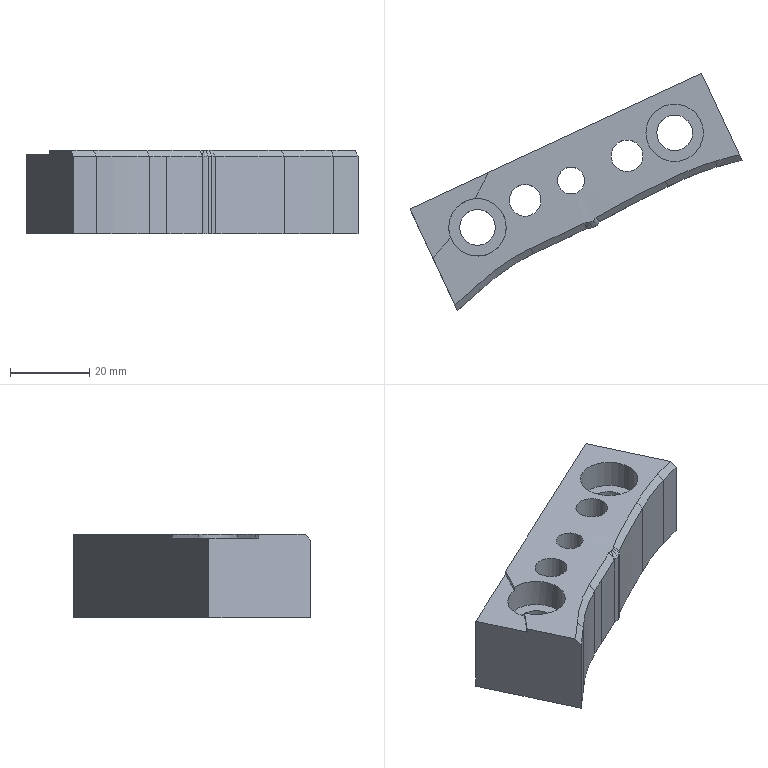Part | NX | features 23 2 | 1 solid | 38 faces | box 83.645 x 59.809 x 21 mm | volume 32912 mm3 | cylinder 17 | plane 10 | cone 9 | spline 2 | commonest cylinder face diameters 4.4 x2 8.001 x2 9 x2 14.5 x2 6.8 x1 134.826 x1
STEP:
#1=CARTESIAN_POINT('',(1048.407,219.447,-2.5));
#2=VERTEX_POINT('',#1);
#3=CARTESIAN_POINT('',(1041.157,219.447,-2.5));
#4=DIRECTION('',(0.,0.,-1.));
#5=DIRECTION('',(1.,0.,0.));
#6=AXIS2_PLACEMENT_3D('',#3,#4,#5);
#7=CIRCLE('',#6,7.25);
#8=EDGE_CURVE('',#2,#2,#7,.T.);
#9=ORIENTED_EDGE('',*,*,#8,.T.);
#10=EDGE_LOOP('',(#9));
#11=FACE_BOUND('',#10,.T.);
#12=CARTESIAN_POINT('',(990.822,202.859,-2.5));
#13=VERTEX_POINT('',#12);
#14=CARTESIAN_POINT('',(984.674,193.131,-2.5));
#15=VERTEX_POINT('',#14);
#16=CARTESIAN_POINT('',(991.477,195.638,-2.5));
#17=DIRECTION('',(0.,0.,-1.));
#18=DIRECTION('',(1.,0.,0.));
#19=AXIS2_PLACEMENT_3D('',#16,#17,#18);
#20=CIRCLE('',#19,7.25);
#21=EDGE_CURVE('',#13,#15,#20,.T.);
#22=ORIENTED_EDGE('',*,*,#21,.T.);
#23=CARTESIAN_POINT('',(980.932,188.619,-2.5));
#24=VERTEX_POINT('',#23);
#25=CARTESIAN_POINT('',(930.965,233.873,-2.5));
#26=DIRECTION('',(0.,0.,-1.));
#27=DIRECTION('',(1.,0.,0.));
#28=AXIS2_PLACEMENT_3D('',#25,#26,#27);
#29=CIRCLE('',#28,67.413);
#30=EDGE_CURVE('',#15,#24,#29,.T.);
#31=ORIENTED_EDGE('',*,*,#30,.T.);
#32=CARTESIAN_POINT('',(980.302,187.761,-2.5));
#33=VERTEX_POINT('',#32);
#34=CARTESIAN_POINT('',(923.807,229.9,-2.5));
#35=DIRECTION('',(0.,0.,-1.));
#36=DIRECTION('',(1.,0.,0.));
#37=AXIS2_PLACEMENT_3D('',#34,#35,#36);
#38=CIRCLE('',#37,70.48);
#39=EDGE_CURVE('',#24,#33,#38,.T.);
#40=ORIENTED_EDGE('',*,*,#39,.T.);
#41=CARTESIAN_POINT('',(985.747,176.055,-2.5));
#42=VERTEX_POINT('',#41);
#43=CARTESIAN_POINT('',(976.037,196.931,-2.5));
#44=DIRECTION('',(0.4218,-0.9067,0.));
#45=VECTOR('',#44,1000.);
#46=LINE('',#43,#45);
#47=EDGE_CURVE('',#33,#42,#46,.T.);
#48=ORIENTED_EDGE('',*,*,#47,.T.);
#49=CARTESIAN_POINT('',(991.288,180.902,-2.5));
#50=VERTEX_POINT('',#49);
#51=CARTESIAN_POINT('',(1024.467,209.927,-2.5));
#52=DIRECTION('',(0.7526,0.6584,0.));
#53=VECTOR('',#52,1000.);
#54=LINE('',#51,#53);
#55=EDGE_CURVE('',#42,#50,#54,.T.);
#56=ORIENTED_EDGE('',*,*,#55,.T.);
#57=CARTESIAN_POINT('',(1004.952,190.387,-2.5));
#58=VERTEX_POINT('',#57);
#59=CARTESIAN_POINT('',(1028.917,141.281,-2.5));
#60=DIRECTION('',(0.,0.,1.));
#61=DIRECTION('',(1.,0.,0.));
#62=AXIS2_PLACEMENT_3D('',#59,#60,#61);
#63=CIRCLE('',#62,54.642);
#64=EDGE_CURVE('',#58,#50,#63,.T.);
#65=ORIENTED_EDGE('',*,*,#64,.F.);
#66=CARTESIAN_POINT('',(1018.301,196.697,-2.5));
#67=VERTEX_POINT('',#66);
#68=CARTESIAN_POINT('',(820.757,597.362,-2.5));
#69=DIRECTION('',(0.,0.,1.));
#70=DIRECTION('',(1.,0.,0.));
#71=AXIS2_PLACEMENT_3D('',#68,#69,#70);
#72=CIRCLE('',#71,446.718);
#73=EDGE_CURVE('',#58,#67,#72,.T.);
#74=ORIENTED_EDGE('',*,*,#73,.T.);
#75=CARTESIAN_POINT('',(1019.215,196.786,-2.5));
#76=VERTEX_POINT('',#75);
#77=CARTESIAN_POINT('',(1018.876,195.531,-2.5));
#78=DIRECTION('',(0.,0.,1.));
#79=DIRECTION('',(1.,0.,0.));
#80=AXIS2_PLACEMENT_3D('',#77,#78,#79);
#81=CIRCLE('',#80,1.3);
#82=EDGE_CURVE('',#76,#67,#81,.T.);
#83=ORIENTED_EDGE('',*,*,#82,.F.);
#84=CARTESIAN_POINT('',(1019.709,196.836,-2.5));
#85=VERTEX_POINT('',#84);
#86=CARTESIAN_POINT('',(1019.397,197.462,-2.5));
#87=DIRECTION('',(0.,0.,1.));
#88=DIRECTION('',(1.,0.,0.));
#89=AXIS2_PLACEMENT_3D('',#86,#87,#88);
#90=CIRCLE('',#89,0.7);
#91=EDGE_CURVE('',#76,#85,#90,.T.);
#92=ORIENTED_EDGE('',*,*,#91,.T.);
#93=CARTESIAN_POINT('',(1020.605,197.282,-2.5));
#94=VERTEX_POINT('',#93);
#95=CARTESIAN_POINT('',(820.757,597.362,-2.5));
#96=DIRECTION('',(0.,0.,1.));
#97=DIRECTION('',(1.,0.,0.));
#98=AXIS2_PLACEMENT_3D('',#95,#96,#97);
#99=CIRCLE('',#98,447.218);
#100=EDGE_CURVE('',#85,#94,#99,.T.);
#101=ORIENTED_EDGE('',*,*,#100,.T.);
#102=CARTESIAN_POINT('',(1021.086,197.957,-2.6));
#103=VERTEX_POINT('',#102);
#104=CARTESIAN_POINT('',(1020.292,197.908,-2.5));
#105=DIRECTION('',(0.,0.,1.));
#106=DIRECTION('',(1.,0.,0.));
#107=AXIS2_PLACEMENT_3D('',#104,#105,#106);
#108=CIRCLE('',#107,0.7);
#109=EDGE_CURVE('',#94,#103,#108,.T.);
#110=ORIENTED_EDGE('',*,*,#109,.T.);
#111=CARTESIAN_POINT('',(1038.834,207.286,-2.5));
#112=VERTEX_POINT('',#111);
#113=CARTESIAN_POINT('',(1180.058,-86.42,-2.5));
#114=DIRECTION('',(0.,0.,1.));
#115=DIRECTION('',(1.,0.,0.));
#116=AXIS2_PLACEMENT_3D('',#113,#114,#115);
#117=CIRCLE('',#116,325.895);
#118=EDGE_CURVE('',#112,#103,#117,.T.);
#119=ORIENTED_EDGE('',*,*,#118,.F.);
#120=CARTESIAN_POINT('',(1051.413,212.327,-2.5));
#121=VERTEX_POINT('',#120);
#122=CARTESIAN_POINT('',(1075.831,133.183,-2.5));
#123=DIRECTION('',(0.,0.,1.));
#124=DIRECTION('',(1.,0.,0.));
#125=AXIS2_PLACEMENT_3D('',#122,#123,#124);
#126=CIRCLE('',#125,82.826);
#127=EDGE_CURVE('',#121,#112,#126,.T.);
#128=ORIENTED_EDGE('',*,*,#127,.F.);
#129=CARTESIAN_POINT('',(1057.475,213.906,-2.5));
#130=VERTEX_POINT('',#129);
#131=CARTESIAN_POINT('',(1086.33,90.693,-2.5));
#132=DIRECTION('',(0.,0.,1.));
#133=DIRECTION('',(1.,0.,0.));
#134=AXIS2_PLACEMENT_3D('',#131,#132,#133);
#135=CIRCLE('',#134,126.547);
#136=EDGE_CURVE('',#130,#121,#135,.T.);
#137=ORIENTED_EDGE('',*,*,#136,.F.);
#138=CARTESIAN_POINT('',(1047.92,234.447,-2.5));
#139=VERTEX_POINT('',#138);
#140=CARTESIAN_POINT('',(1051.784,226.14,-2.5));
#141=DIRECTION('',(-0.4218,0.9067,0.));
#142=VECTOR('',#141,1000.);
#143=LINE('',#140,#142);
#144=EDGE_CURVE('',#130,#139,#143,.T.);
#145=ORIENTED_EDGE('',*,*,#144,.T.);
#146=CARTESIAN_POINT('',(994.242,209.479,-2.5));
#147=VERTEX_POINT('',#146);
#148=CARTESIAN_POINT('',(1076.358,247.675,-2.5));
#149=DIRECTION('',(-0.9067,-0.4218,0.));
#150=VECTOR('',#149,1000.);
#151=LINE('',#148,#150);
#152=EDGE_CURVE('',#139,#147,#151,.T.);
#153=ORIENTED_EDGE('',*,*,#152,.T.);
#154=CARTESIAN_POINT('',(785.133,313.29,-2.5));
#155=DIRECTION('',(0.,0.,-1.));
#156=DIRECTION('',(1.,0.,0.));
#157=AXIS2_PLACEMENT_3D('',#154,#155,#156);
#158=CIRCLE('',#157,233.459);
#159=EDGE_CURVE('',#147,#13,#158,.T.);
#160=ORIENTED_EDGE('',*,*,#159,.T.);
#161=EDGE_LOOP('',(#22,#31,#40,#48,#56,#65,#74,#83,#92,#101,#110,#119,#128,#137,#145,#153,#160));
#162=FACE_BOUND('',#161,.T.);
#163=CARTESIAN_POINT('',(1007.477,202.447,-2.5));
#164=VERTEX_POINT('',#163);
#165=CARTESIAN_POINT('',(1003.477,202.447,-2.5));
#166=DIRECTION('',(0.,0.,-1.));
#167=DIRECTION('',(1.,0.,0.));
#168=AXIS2_PLACEMENT_3D('',#165,#166,#167);
#169=CIRCLE('',#168,4.);
#170=EDGE_CURVE('',#164,#164,#169,.T.);
#171=ORIENTED_EDGE('',*,*,#170,.T.);
#172=EDGE_LOOP('',(#171));
#173=FACE_BOUND('',#172,.T.);
#174=CARTESIAN_POINT('',(1033.158,213.638,-2.5));
#175=VERTEX_POINT('',#174);
#176=CARTESIAN_POINT('',(1029.157,213.638,-2.5));
#177=DIRECTION('',(0.,0.,-1.));
#178=DIRECTION('',(1.,0.,0.));
#179=AXIS2_PLACEMENT_3D('',#176,#177,#178);
#180=CIRCLE('',#179,4.);
#181=EDGE_CURVE('',#175,#175,#180,.T.);
#182=ORIENTED_EDGE('',*,*,#181,.T.);
#183=EDGE_LOOP('',(#182));
#184=FACE_BOUND('',#183,.T.);
#185=CARTESIAN_POINT('',(1018.449,207.41,-2.5));
#186=VERTEX_POINT('',#185);
#187=CARTESIAN_POINT('',(1015.049,207.41,-2.5));
#188=DIRECTION('',(0.,0.,1.));
#189=DIRECTION('',(1.,0.,0.));
#190=AXIS2_PLACEMENT_3D('',#187,#188,#189);
#191=CIRCLE('',#190,3.4);
#192=EDGE_CURVE('',#186,#186,#191,.T.);
#193=ORIENTED_EDGE('',*,*,#192,.F.);
#194=EDGE_LOOP('',(#193));
#195=FACE_BOUND('',#194,.T.);
#196=CARTESIAN_POINT('',(1166.5,279.5,-2.5));
#197=DIRECTION('',(0.,0.,1.));
#198=DIRECTION('',(-1.,0.,0.));
#199=AXIS2_PLACEMENT_3D('',#196,#197,#198);
#200=PLANE('',#199);
#201=ADVANCED_FACE('',(#11,#162,#173,#184,#195),#200,.T.);
#202=CARTESIAN_POINT('',(1009.921,191.018,-23.5));
#203=VERTEX_POINT('',#202);
#204=CARTESIAN_POINT('',(1005.59,189.03,-23.5));
#205=VERTEX_POINT('',#204);
#206=CARTESIAN_POINT('',(1009.921,191.018,-23.5));
#207=CARTESIAN_POINT('',(1008.481,190.347,-23.5));
#208=CARTESIAN_POINT('',(1007.037,189.685,-23.5));
#209=CARTESIAN_POINT('',(1005.59,189.03,-23.5));
#210=(BOUNDED_CURVE()B_SPLINE_CURVE(3,(#206,#207,#208,#209),.UNSPECIFIED.,.F.,.F.)B_SPLINE_CURVE_WITH_KNOTS((4,4),(0.,1.),.PIECEWISE_BEZIER_KNOTS.)CURVE()GEOMETRIC_REPRESENTATION_ITEM()RATIONAL_B_SPLINE_CURVE((1.,1.,1.,1.))REPRESENTATION_ITEM(''));
#211=EDGE_CURVE('',#203,#205,#210,.T.);
#212=ORIENTED_EDGE('',*,*,#211,.F.);
#213=CARTESIAN_POINT('',(1009.921,191.018,-4.));
#214=VERTEX_POINT('',#213);
#215=CARTESIAN_POINT('',(1009.921,191.018,-43.));
#216=DIRECTION('',(0.,0.,-1.));
#217=VECTOR('',#216,1000.);
#218=LINE('',#215,#217);
#219=EDGE_CURVE('',#214,#203,#218,.T.);
#220=ORIENTED_EDGE('',*,*,#219,.F.);
#221=CARTESIAN_POINT('',(1005.59,189.03,-4.));
#222=VERTEX_POINT('',#221);
#223=CARTESIAN_POINT('',(820.757,597.362,-4.));
#224=DIRECTION('',(0.,0.,-1.));
#225=DIRECTION('',(-1.,0.,0.));
#226=AXIS2_PLACEMENT_3D('',#223,#224,#225);
#227=CIRCLE('',#226,448.218);
#228=EDGE_CURVE('',#214,#222,#227,.T.);
#229=ORIENTED_EDGE('',*,*,#228,.T.);
#230=CARTESIAN_POINT('',(1005.59,189.03,-43.));
#231=DIRECTION('',(0.,0.,1.));
#232=VECTOR('',#231,1000.);
#233=LINE('',#230,#232);
#234=EDGE_CURVE('',#205,#222,#233,.T.);
#235=ORIENTED_EDGE('',*,*,#234,.F.);
#236=EDGE_LOOP('',(#212,#220,#229,#235));
#237=FACE_BOUND('',#236,.T.);
#238=CARTESIAN_POINT('',(1005.59,189.03,-23.5));
#239=CARTESIAN_POINT('',(1005.59,189.03,-4.));
#240=CARTESIAN_POINT('',(1007.037,189.685,-23.5));
#241=CARTESIAN_POINT('',(1007.037,189.685,-4.));
#242=CARTESIAN_POINT('',(1008.481,190.347,-23.5));
#243=CARTESIAN_POINT('',(1008.481,190.347,-4.));
#244=CARTESIAN_POINT('',(1009.921,191.018,-23.5));
#245=CARTESIAN_POINT('',(1009.921,191.018,-4.));
#246=B_SPLINE_SURFACE_WITH_KNOTS('',3,1,((#238,#239),(#240,#241),(#242,#243),(#244,#245)),.SURF_OF_LINEAR_EXTRUSION.,.F.,.F.,.F.,(4,4),(2,2),(0.,1.),(0.,1.),.PIECEWISE_BEZIER_KNOTS.);
#247=ADVANCED_FACE('',(#237),#246,.T.);
#248=CARTESIAN_POINT('',(1018.899,195.319,-4.));
#249=VERTEX_POINT('',#248);
#250=CARTESIAN_POINT('',(820.757,597.362,-4.));
#251=DIRECTION('',(0.,0.,-1.));
#252=DIRECTION('',(-1.,0.,0.));
#253=AXIS2_PLACEMENT_3D('',#250,#251,#252);
#254=CIRCLE('',#253,448.218);
#255=EDGE_CURVE('',#249,#214,#254,.T.);
#256=ORIENTED_EDGE('',*,*,#255,.T.);
#257=ORIENTED_EDGE('',*,*,#219,.T.);
#258=CARTESIAN_POINT('',(1018.899,195.319,-23.5));
#259=VERTEX_POINT('',#258);
#260=CARTESIAN_POINT('',(820.757,597.362,-23.5));
#261=DIRECTION('',(0.,0.,1.));
#262=DIRECTION('',(-1.,0.,0.));
#263=AXIS2_PLACEMENT_3D('',#260,#261,#262);
#264=CIRCLE('',#263,448.218);
#265=EDGE_CURVE('',#203,#259,#264,.T.);
#266=ORIENTED_EDGE('',*,*,#265,.T.);
#267=CARTESIAN_POINT('',(1018.899,195.319,-43.));
#268=DIRECTION('',(0.,0.,1.));
#269=VECTOR('',#268,1000.);
#270=LINE('',#267,#269);
#271=EDGE_CURVE('',#259,#249,#270,.T.);
#272=ORIENTED_EDGE('',*,*,#271,.T.);
#273=EDGE_LOOP('',(#256,#257,#266,#272));
#274=FACE_BOUND('',#273,.T.);
#275=CARTESIAN_POINT('',(820.757,597.362,-43.));
#276=DIRECTION('',(0.,0.,1.));
#277=DIRECTION('',(-1.,0.,0.));
#278=AXIS2_PLACEMENT_3D('',#275,#276,#277);
#279=CYLINDRICAL_SURFACE('',#278,448.218);
#280=ADVANCED_FACE('',(#274),#279,.T.);
#281=CARTESIAN_POINT('',(1020.38,195.494,-4.));
#282=VERTEX_POINT('',#281);
#283=CARTESIAN_POINT('',(1019.397,197.462,-4.));
#284=DIRECTION('',(0.,0.,-1.));
#285=DIRECTION('',(-1.,0.,0.));
#286=AXIS2_PLACEMENT_3D('',#283,#284,#285);
#287=CIRCLE('',#286,2.2);
#288=EDGE_CURVE('',#282,#249,#287,.T.);
#289=ORIENTED_EDGE('',*,*,#288,.T.);
#290=ORIENTED_EDGE('',*,*,#271,.F.);
#291=CARTESIAN_POINT('',(1020.38,195.494,-23.5));
#292=VERTEX_POINT('',#291);
#293=CARTESIAN_POINT('',(1019.397,197.462,-23.5));
#294=DIRECTION('',(0.,0.,-1.));
#295=DIRECTION('',(-1.,0.,0.));
#296=AXIS2_PLACEMENT_3D('',#293,#294,#295);
#297=CIRCLE('',#296,2.2);
#298=EDGE_CURVE('',#292,#259,#297,.T.);
#299=ORIENTED_EDGE('',*,*,#298,.F.);
#300=CARTESIAN_POINT('',(1020.38,195.494,-43.));
#301=DIRECTION('',(0.,0.,1.));
#302=VECTOR('',#301,1000.);
#303=LINE('',#300,#302);
#304=EDGE_CURVE('',#292,#282,#303,.T.);
#305=ORIENTED_EDGE('',*,*,#304,.T.);
#306=EDGE_LOOP('',(#289,#290,#299,#305));
#307=FACE_BOUND('',#306,.T.);
#308=CARTESIAN_POINT('',(1019.397,197.462,-43.));
#309=DIRECTION('',(0.,0.,1.));
#310=DIRECTION('',(-1.,0.,0.));
#311=AXIS2_PLACEMENT_3D('',#308,#309,#310);
#312=CYLINDRICAL_SURFACE('',#311,2.2);
#313=ADVANCED_FACE('',(#307),#312,.T.);
#314=CARTESIAN_POINT('',(1021.275,195.94,-4.));
#315=VERTEX_POINT('',#314);
#316=CARTESIAN_POINT('',(820.757,597.362,-4.));
#317=DIRECTION('',(0.,0.,-1.));
#318=DIRECTION('',(-1.,0.,0.));
#319=AXIS2_PLACEMENT_3D('',#316,#317,#318);
#320=CIRCLE('',#319,448.718);
#321=EDGE_CURVE('',#315,#282,#320,.T.);
#322=ORIENTED_EDGE('',*,*,#321,.T.);
#323=ORIENTED_EDGE('',*,*,#304,.F.);
#324=CARTESIAN_POINT('',(1021.275,195.94,-23.5));
#325=VERTEX_POINT('',#324);
#326=CARTESIAN_POINT('',(820.757,597.362,-23.5));
#327=DIRECTION('',(0.,0.,1.));
#328=DIRECTION('',(-1.,0.,0.));
#329=AXIS2_PLACEMENT_3D('',#326,#327,#328);
#330=CIRCLE('',#329,448.718);
#331=EDGE_CURVE('',#292,#325,#330,.T.);
#332=ORIENTED_EDGE('',*,*,#331,.T.);
#333=CARTESIAN_POINT('',(1021.275,195.94,-43.));
#334=DIRECTION('',(0.,0.,1.));
#335=VECTOR('',#334,1000.);
#336=LINE('',#333,#335);
#337=EDGE_CURVE('',#325,#315,#336,.T.);
#338=ORIENTED_EDGE('',*,*,#337,.T.);
#339=EDGE_LOOP('',(#322,#323,#332,#338));
#340=FACE_BOUND('',#339,.T.);
#341=CARTESIAN_POINT('',(820.757,597.362,-43.));
#342=DIRECTION('',(0.,0.,1.));
#343=DIRECTION('',(-1.,0.,0.));
#344=AXIS2_PLACEMENT_3D('',#341,#342,#343);
#345=CYLINDRICAL_SURFACE('',#344,448.718);
#346=ADVANCED_FACE('',(#340),#345,.T.);
#347=CARTESIAN_POINT('',(1022.284,197.08,-3.958));
#348=VERTEX_POINT('',#347);
#349=CARTESIAN_POINT('',(1020.292,197.908,-4.));
#350=DIRECTION('',(0.,0.,-1.));
#351=DIRECTION('',(-1.,0.,0.));
#352=AXIS2_PLACEMENT_3D('',#349,#350,#351);
#353=CIRCLE('',#352,2.2);
#354=EDGE_CURVE('',#348,#315,#353,.T.);
#355=ORIENTED_EDGE('',*,*,#354,.T.);
#356=ORIENTED_EDGE('',*,*,#337,.F.);
#357=CARTESIAN_POINT('',(1022.312,197.038,-23.5));
#358=VERTEX_POINT('',#357);
#359=CARTESIAN_POINT('',(1020.292,197.908,-23.5));
#360=DIRECTION('',(0.,0.,-1.));
#361=DIRECTION('',(-1.,0.,0.));
#362=AXIS2_PLACEMENT_3D('',#359,#360,#361);
#363=CIRCLE('',#362,2.2);
#364=EDGE_CURVE('',#358,#325,#363,.T.);
#365=ORIENTED_EDGE('',*,*,#364,.F.);
#366=CARTESIAN_POINT('',(1022.312,197.038,-43.));
#367=DIRECTION('',(0.,0.,1.));
#368=VECTOR('',#367,1000.);
#369=LINE('',#366,#368);
#370=EDGE_CURVE('',#358,#348,#369,.T.);
#371=ORIENTED_EDGE('',*,*,#370,.T.);
#372=EDGE_LOOP('',(#355,#356,#365,#371));
#373=FACE_BOUND('',#372,.T.);
#374=CARTESIAN_POINT('',(1020.292,197.908,-43.));
#375=DIRECTION('',(0.,0.,1.));
#376=DIRECTION('',(-1.,0.,0.));
#377=AXIS2_PLACEMENT_3D('',#374,#375,#376);
#378=CYLINDRICAL_SURFACE('',#377,2.2);
#379=ADVANCED_FACE('',(#373),#378,.T.);
#380=ORIENTED_EDGE('',*,*,#370,.F.);
#381=CARTESIAN_POINT('',(1039.494,205.939,-23.5));
#382=VERTEX_POINT('',#381);
#383=CARTESIAN_POINT('',(1180.058,-86.42,-23.5));
#384=DIRECTION('',(0.,0.,-1.));
#385=DIRECTION('',(-1.,0.,0.));
#386=AXIS2_PLACEMENT_3D('',#383,#384,#385);
#387=CIRCLE('',#386,324.395);
#388=EDGE_CURVE('',#358,#382,#387,.T.);
#389=ORIENTED_EDGE('',*,*,#388,.T.);
#390=CARTESIAN_POINT('',(1039.494,205.939,-4.));
#391=VERTEX_POINT('',#390);
#392=CARTESIAN_POINT('',(1039.494,205.939,-43.));
#393=DIRECTION('',(0.,0.,1.));
#394=VECTOR('',#393,1000.);
#395=LINE('',#392,#394);
#396=EDGE_CURVE('',#382,#391,#395,.T.);
#397=ORIENTED_EDGE('',*,*,#396,.T.);
#398=CARTESIAN_POINT('',(1180.058,-86.42,-4.));
#399=DIRECTION('',(0.,0.,1.));
#400=DIRECTION('',(-1.,0.,0.));
#401=AXIS2_PLACEMENT_3D('',#398,#399,#400);
#402=CIRCLE('',#401,324.395);
#403=EDGE_CURVE('',#391,#348,#402,.T.);
#404=ORIENTED_EDGE('',*,*,#403,.T.);
#405=EDGE_LOOP('',(#380,#389,#397,#404));
#406=FACE_BOUND('',#405,.T.);
#407=CARTESIAN_POINT('',(1180.058,-86.42,-43.));
#408=DIRECTION('',(0.,0.,1.));
#409=DIRECTION('',(-1.,0.,0.));
#410=AXIS2_PLACEMENT_3D('',#407,#408,#409);
#411=CYLINDRICAL_SURFACE('',#410,324.395);
#412=ADVANCED_FACE('',(#406),#411,.F.);
#413=ORIENTED_EDGE('',*,*,#396,.F.);
#414=CARTESIAN_POINT('',(1051.841,210.889,-23.5));
#415=VERTEX_POINT('',#414);
#416=CARTESIAN_POINT('',(1075.831,133.183,-23.5));
#417=DIRECTION('',(0.,0.,1.));
#418=DIRECTION('',(-1.,0.,0.));
#419=AXIS2_PLACEMENT_3D('',#416,#417,#418);
#420=CIRCLE('',#419,81.326);
#421=EDGE_CURVE('',#415,#382,#420,.T.);
#422=ORIENTED_EDGE('',*,*,#421,.F.);
#423=CARTESIAN_POINT('',(1051.841,210.889,-4.));
#424=VERTEX_POINT('',#423);
#425=CARTESIAN_POINT('',(1051.841,210.889,-43.));
#426=DIRECTION('',(0.,0.,-1.));
#427=VECTOR('',#426,1000.);
#428=LINE('',#425,#427);
#429=EDGE_CURVE('',#424,#415,#428,.T.);
#430=ORIENTED_EDGE('',*,*,#429,.F.);
#431=CARTESIAN_POINT('',(1075.831,133.183,-4.));
#432=DIRECTION('',(0.,0.,1.));
#433=DIRECTION('',(-1.,0.,0.));
#434=AXIS2_PLACEMENT_3D('',#431,#432,#433);
#435=CIRCLE('',#434,81.326);
#436=EDGE_CURVE('',#424,#391,#435,.T.);
#437=ORIENTED_EDGE('',*,*,#436,.T.);
#438=EDGE_LOOP('',(#413,#422,#430,#437));
#439=FACE_BOUND('',#438,.T.);
#440=CARTESIAN_POINT('',(1075.831,133.183,-43.));
#441=DIRECTION('',(0.,0.,1.));
#442=DIRECTION('',(-1.,0.,0.));
#443=AXIS2_PLACEMENT_3D('',#440,#441,#442);
#444=CYLINDRICAL_SURFACE('',#443,81.326);
#445=ADVANCED_FACE('',(#439),#444,.F.);
#446=ORIENTED_EDGE('',*,*,#152,.F.);
#447=CARTESIAN_POINT('',(1047.92,234.447,-23.5));
#448=VERTEX_POINT('',#447);
#449=CARTESIAN_POINT('',(1047.92,234.447,-13.));
#450=DIRECTION('',(0.,0.,-1.));
#451=VECTOR('',#450,1000.);
#452=LINE('',#449,#451);
#453=EDGE_CURVE('',#139,#448,#452,.T.);
#454=ORIENTED_EDGE('',*,*,#453,.T.);
#455=CARTESIAN_POINT('',(974.477,200.285,-23.5));
#456=VERTEX_POINT('',#455);
#457=CARTESIAN_POINT('',(1076.358,247.675,-23.5));
#458=DIRECTION('',(0.9067,0.4218,0.));
#459=VECTOR('',#458,1000.);
#460=LINE('',#457,#459);
#461=EDGE_CURVE('',#456,#448,#460,.T.);
#462=ORIENTED_EDGE('',*,*,#461,.F.);
#463=CARTESIAN_POINT('',(974.477,200.285,-3.5));
#464=VERTEX_POINT('',#463);
#465=CARTESIAN_POINT('',(974.477,200.285,0.));
#466=DIRECTION('',(0.,0.,-1.));
#467=VECTOR('',#466,1000.);
#468=LINE('',#465,#467);
#469=EDGE_CURVE('',#464,#456,#468,.T.);
#470=ORIENTED_EDGE('',*,*,#469,.F.);
#471=CARTESIAN_POINT('',(994.242,209.479,-3.5));
#472=VERTEX_POINT('',#471);
#473=CARTESIAN_POINT('',(1076.358,247.675,-3.5));
#474=DIRECTION('',(0.9067,0.4218,0.));
#475=VECTOR('',#474,1000.);
#476=LINE('',#473,#475);
#477=EDGE_CURVE('',#464,#472,#476,.T.);
#478=ORIENTED_EDGE('',*,*,#477,.T.);
#479=CARTESIAN_POINT('',(994.242,209.479,-2.5));
#480=DIRECTION('',(0.,0.,1.));
#481=VECTOR('',#480,1000.);
#482=LINE('',#479,#481);
#483=EDGE_CURVE('',#472,#147,#482,.T.);
#484=ORIENTED_EDGE('',*,*,#483,.T.);
#485=EDGE_LOOP('',(#446,#454,#462,#470,#478,#484));
#486=FACE_BOUND('',#485,.T.);
#487=CARTESIAN_POINT('',(1076.358,247.675,0.));
#488=DIRECTION('',(-0.4218,0.9067,0.));
#489=DIRECTION('',(0.,0.,1.));
#490=AXIS2_PLACEMENT_3D('',#487,#488,#489);
#491=PLANE('',#490);
#492=ADVANCED_FACE('',(#486),#491,.T.);
#493=CARTESIAN_POINT('',(1051.598,211.704,-3.15));
#494=DIRECTION('',(-0.2018,0.6777,0.7071));
#495=VECTOR('',#494,1000.);
#496=LINE('',#493,#495);
#497=EDGE_CURVE('',#424,#121,#496,.T.);
#498=ORIENTED_EDGE('',*,*,#497,.F.);
#499=CARTESIAN_POINT('',(1058.121,212.516,-4.));
#500=VERTEX_POINT('',#499);
#501=CARTESIAN_POINT('',(1086.33,90.693,-4.));
#502=DIRECTION('',(0.,0.,-1.));
#503=DIRECTION('',(1.,0.,0.));
#504=AXIS2_PLACEMENT_3D('',#501,#502,#503);
#505=CIRCLE('',#504,125.047);
#506=EDGE_CURVE('',#424,#500,#505,.T.);
#507=ORIENTED_EDGE('',*,*,#506,.T.);
#508=CARTESIAN_POINT('',(1057.475,213.906,-2.5));
#509=CARTESIAN_POINT('',(1057.69,213.443,-3.));
#510=CARTESIAN_POINT('',(1057.906,212.98,-3.5));
#511=CARTESIAN_POINT('',(1058.121,212.516,-4.));
#512=B_SPLINE_CURVE_WITH_KNOTS('',3,(#508,#509,#510,#511),.UNSPECIFIED.,.F.,.F.,(4,4),(0.,1.),.PIECEWISE_BEZIER_KNOTS.);
#513=EDGE_CURVE('',#130,#500,#512,.T.);
#514=ORIENTED_EDGE('',*,*,#513,.F.);
#515=ORIENTED_EDGE('',*,*,#136,.T.);
#516=EDGE_LOOP('',(#498,#507,#514,#515));
#517=FACE_BOUND('',#516,.T.);
#518=CARTESIAN_POINT('',(1086.33,90.693,-3.5));
#519=DIRECTION('',(0.,0.,1.));
#520=DIRECTION('',(1.,0.,0.));
#521=AXIS2_PLACEMENT_3D('',#518,#519,#520);
#522=CONICAL_SURFACE('',#521,125.547,0.7854);
#523=ADVANCED_FACE('',(#517),#522,.F.);
#524=ORIENTED_EDGE('',*,*,#436,.F.);
#525=ORIENTED_EDGE('',*,*,#497,.T.);
#526=ORIENTED_EDGE('',*,*,#127,.T.);
#527=CARTESIAN_POINT('',(1039.12,206.703,-3.15));
#528=DIRECTION('',(-0.3112,0.635,0.7071));
#529=VECTOR('',#528,1000.);
#530=LINE('',#527,#529);
#531=EDGE_CURVE('',#391,#112,#530,.T.);
#532=ORIENTED_EDGE('',*,*,#531,.F.);
#533=EDGE_LOOP('',(#524,#525,#526,#532));
#534=FACE_BOUND('',#533,.T.);
#535=CARTESIAN_POINT('',(1075.831,133.183,-3.5));
#536=DIRECTION('',(0.,0.,1.));
#537=DIRECTION('',(1.,0.,0.));
#538=AXIS2_PLACEMENT_3D('',#535,#536,#537);
#539=CONICAL_SURFACE('',#538,81.826,0.7854);
#540=ADVANCED_FACE('',(#534),#539,.F.);
#541=ORIENTED_EDGE('',*,*,#118,.T.);
#542=CARTESIAN_POINT('',(1022.278,197.069,-3.956));
#543=CARTESIAN_POINT('',(1021.914,197.395,-3.494));
#544=CARTESIAN_POINT('',(1021.542,197.714,-3.035));
#545=CARTESIAN_POINT('',(1021.089,197.96,-2.599));
#546=B_SPLINE_CURVE_WITH_KNOTS('',3,(#542,#543,#544,#545),.UNSPECIFIED.,.F.,.F.,(4,4),(0.000000026,0.002012),.UNSPECIFIED.);
#547=EDGE_CURVE('',#348,#103,#546,.T.);
#548=ORIENTED_EDGE('',*,*,#547,.F.);
#549=ORIENTED_EDGE('',*,*,#403,.F.);
#550=ORIENTED_EDGE('',*,*,#531,.T.);
#551=EDGE_LOOP('',(#541,#548,#549,#550));
#552=FACE_BOUND('',#551,.T.);
#553=CARTESIAN_POINT('',(1180.058,-86.42,-3.5));
#554=DIRECTION('',(0.,0.,1.));
#555=DIRECTION('',(1.,0.,0.));
#556=AXIS2_PLACEMENT_3D('',#553,#554,#555);
#557=CONICAL_SURFACE('',#556,324.895,0.7854);
#558=ADVANCED_FACE('',(#552),#557,.F.);
#559=ORIENTED_EDGE('',*,*,#547,.T.);
#560=ORIENTED_EDGE('',*,*,#109,.F.);
#561=CARTESIAN_POINT('',(1021.051,196.387,-3.5));
#562=DIRECTION('',(-0.316,0.6326,0.7071));
#563=VECTOR('',#562,1000.);
#564=LINE('',#561,#563);
#565=EDGE_CURVE('',#315,#94,#564,.T.);
#566=ORIENTED_EDGE('',*,*,#565,.F.);
#567=ORIENTED_EDGE('',*,*,#354,.F.);
#568=EDGE_LOOP('',(#559,#560,#566,#567));
#569=FACE_BOUND('',#568,.T.);
#570=CARTESIAN_POINT('',(1020.292,197.908,-3.5));
#571=DIRECTION('',(0.,0.,-1.));
#572=DIRECTION('',(-1.,0.,0.));
#573=AXIS2_PLACEMENT_3D('',#570,#571,#572);
#574=CONICAL_SURFACE('',#573,1.7,0.7854);
#575=ADVANCED_FACE('',(#569),#574,.T.);
#576=ORIENTED_EDGE('',*,*,#565,.T.);
#577=ORIENTED_EDGE('',*,*,#100,.F.);
#578=CARTESIAN_POINT('',(1020.156,195.941,-3.5));
#579=DIRECTION('',(-0.316,0.6326,0.7071));
#580=VECTOR('',#579,1000.);
#581=LINE('',#578,#580);
#582=EDGE_CURVE('',#282,#85,#581,.T.);
#583=ORIENTED_EDGE('',*,*,#582,.F.);
#584=ORIENTED_EDGE('',*,*,#321,.F.);
#585=EDGE_LOOP('',(#576,#577,#583,#584));
#586=FACE_BOUND('',#585,.T.);
#587=CARTESIAN_POINT('',(820.757,597.362,-3.5));
#588=DIRECTION('',(0.,0.,-1.));
#589=DIRECTION('',(-1.,0.,0.));
#590=AXIS2_PLACEMENT_3D('',#587,#588,#589);
#591=CONICAL_SURFACE('',#590,448.218,0.7854);
#592=ADVANCED_FACE('',(#586),#591,.T.);
#593=ORIENTED_EDGE('',*,*,#582,.T.);
#594=ORIENTED_EDGE('',*,*,#91,.F.);
#595=CARTESIAN_POINT('',(1018.876,195.531,-3.8));
#596=VERTEX_POINT('',#595);
#597=CARTESIAN_POINT('',(1018.954,195.821,-3.5));
#598=DIRECTION('',(0.184,0.6828,0.7071));
#599=VECTOR('',#598,1000.);
#600=LINE('',#597,#599);
#601=EDGE_CURVE('',#596,#76,#600,.T.);
#602=ORIENTED_EDGE('',*,*,#601,.F.);
#603=CARTESIAN_POINT('',(1018.899,195.319,-4.));
#604=CARTESIAN_POINT('',(1018.891,195.389,-3.933));
#605=CARTESIAN_POINT('',(1018.883,195.46,-3.867));
#606=CARTESIAN_POINT('',(1018.876,195.531,-3.8));
#607=B_SPLINE_CURVE_WITH_KNOTS('',3,(#603,#604,#605,#606),.UNSPECIFIED.,.F.,.F.,(4,4),(0.,1.),.PIECEWISE_BEZIER_KNOTS.);
#608=EDGE_CURVE('',#249,#596,#607,.T.);
#609=ORIENTED_EDGE('',*,*,#608,.F.);
#610=ORIENTED_EDGE('',*,*,#288,.F.);
#611=EDGE_LOOP('',(#593,#594,#602,#609,#610));
#612=FACE_BOUND('',#611,.T.);
#613=CARTESIAN_POINT('',(1019.397,197.462,-3.5));
#614=DIRECTION('',(0.,0.,-1.));
#615=DIRECTION('',(-1.,0.,0.));
#616=AXIS2_PLACEMENT_3D('',#613,#614,#615);
#617=CONICAL_SURFACE('',#616,1.7,0.7854);
#618=ADVANCED_FACE('',(#612),#617,.T.);
#619=ORIENTED_EDGE('',*,*,#82,.T.);
#620=CARTESIAN_POINT('',(1018.744,195.8,-3.5));
#621=DIRECTION('',(-0.3127,0.6342,0.7071));
#622=VECTOR('',#621,1000.);
#623=LINE('',#620,#622);
#624=EDGE_CURVE('',#596,#67,#623,.T.);
#625=ORIENTED_EDGE('',*,*,#624,.F.);
#626=ORIENTED_EDGE('',*,*,#601,.T.);
#627=EDGE_LOOP('',(#619,#625,#626));
#628=FACE_BOUND('',#627,.T.);
#629=CARTESIAN_POINT('',(1018.876,195.531,-3.5));
#630=DIRECTION('',(0.,0.,1.));
#631=DIRECTION('',(1.,0.,0.));
#632=AXIS2_PLACEMENT_3D('',#629,#630,#631);
#633=CONICAL_SURFACE('',#632,0.3,0.7854);
#634=ADVANCED_FACE('',(#628),#633,.F.);
#635=ORIENTED_EDGE('',*,*,#228,.F.);
#636=ORIENTED_EDGE('',*,*,#255,.F.);
#637=ORIENTED_EDGE('',*,*,#608,.T.);
#638=ORIENTED_EDGE('',*,*,#624,.T.);
#639=ORIENTED_EDGE('',*,*,#73,.F.);
#640=CARTESIAN_POINT('',(1005.654,188.894,-4.15));
#641=CARTESIAN_POINT('',(1005.621,188.964,-4.073));
#642=CARTESIAN_POINT('',(1005.589,189.033,-3.996));
#643=CARTESIAN_POINT('',(1005.531,189.156,-3.86));
#644=CARTESIAN_POINT('',(1005.505,189.21,-3.801));
#645=CARTESIAN_POINT('',(1005.461,189.305,-3.696));
#646=CARTESIAN_POINT('',(1005.442,189.346,-3.65));
#647=CARTESIAN_POINT('',(1005.407,189.419,-3.57));
#648=CARTESIAN_POINT('',(1005.392,189.45,-3.535));
#649=CARTESIAN_POINT('',(1005.278,189.693,-3.267));
#650=CARTESIAN_POINT('',(1005.179,189.904,-3.033));
#651=CARTESIAN_POINT('',(1005.065,190.147,-2.765));
#652=CARTESIAN_POINT('',(1005.05,190.179,-2.73));
#653=CARTESIAN_POINT('',(1005.015,190.252,-2.649));
#654=CARTESIAN_POINT('',(1004.996,190.293,-2.604));
#655=CARTESIAN_POINT('',(1004.952,190.388,-2.499));
#656=CARTESIAN_POINT('',(1004.926,190.441,-2.44));
#657=CARTESIAN_POINT('',(1004.869,190.564,-2.304));
#658=CARTESIAN_POINT('',(1004.836,190.634,-2.227));
#659=CARTESIAN_POINT('',(1004.803,190.704,-2.15));
#660=B_SPLINE_CURVE_WITH_KNOTS('',3,(#640,#641,#642,#643,#644,#645,#646,#647,#648,#649,#650,#651,#652,#653,#654,#655,#656,#657,#658,#659),.UNSPECIFIED.,.F.,.F.,(4,2,2,2,2,2,2,2,2,4),(0.,0.1154,0.2041,0.2724,0.3249,0.6751,0.7276,0.7959,0.8846,1.),.UNSPECIFIED.);
#661=EDGE_CURVE('',#222,#58,#660,.T.);
#662=ORIENTED_EDGE('',*,*,#661,.F.);
#663=EDGE_LOOP('',(#635,#636,#637,#638,#639,#662));
#664=FACE_BOUND('',#663,.T.);
#665=CARTESIAN_POINT('',(820.757,597.362,-3.5));
#666=DIRECTION('',(0.,0.,-1.));
#667=DIRECTION('',(-1.,0.,0.));
#668=AXIS2_PLACEMENT_3D('',#665,#666,#667);
#669=CONICAL_SURFACE('',#668,447.718,0.7854);
#670=ADVANCED_FACE('',(#664),#669,.T.);
#671=ORIENTED_EDGE('',*,*,#64,.T.);
#672=CARTESIAN_POINT('',(992.299,179.793,-4.));
#673=VERTEX_POINT('',#672);
#674=CARTESIAN_POINT('',(992.4,179.682,-4.15));
#675=CARTESIAN_POINT('',(992.348,179.739,-4.073));
#676=CARTESIAN_POINT('',(992.296,179.796,-3.996));
#677=CARTESIAN_POINT('',(992.204,179.896,-3.86));
#678=CARTESIAN_POINT('',(992.164,179.94,-3.801));
#679=CARTESIAN_POINT('',(992.094,180.018,-3.696));
#680=CARTESIAN_POINT('',(992.063,180.051,-3.65));
#681=CARTESIAN_POINT('',(992.009,180.111,-3.57));
#682=CARTESIAN_POINT('',(991.985,180.137,-3.535));
#683=CARTESIAN_POINT('',(991.805,180.335,-3.267));
#684=CARTESIAN_POINT('',(991.647,180.507,-3.033));
#685=CARTESIAN_POINT('',(991.467,180.706,-2.765));
#686=CARTESIAN_POINT('',(991.443,180.732,-2.73));
#687=CARTESIAN_POINT('',(991.389,180.791,-2.649));
#688=CARTESIAN_POINT('',(991.358,180.825,-2.604));
#689=CARTESIAN_POINT('',(991.288,180.902,-2.499));
#690=CARTESIAN_POINT('',(991.248,180.946,-2.44));
#691=CARTESIAN_POINT('',(991.156,181.046,-2.304));
#692=CARTESIAN_POINT('',(991.104,181.103,-2.227));
#693=CARTESIAN_POINT('',(991.052,181.16,-2.15));
#694=B_SPLINE_CURVE_WITH_KNOTS('',3,(#674,#675,#676,#677,#678,#679,#680,#681,#682,#683,#684,#685,#686,#687,#688,#689,#690,#691,#692,#693),.UNSPECIFIED.,.F.,.F.,(4,2,2,2,2,2,2,2,2,4),(0.,0.1154,0.2041,0.2724,0.3249,0.6751,0.7276,0.7959,0.8846,1.),.UNSPECIFIED.);
#695=EDGE_CURVE('',#673,#50,#694,.T.);
#696=ORIENTED_EDGE('',*,*,#695,.F.);
#697=CARTESIAN_POINT('',(992.299,179.793,-4.));
#698=CARTESIAN_POINT('',(996.239,183.54,-4.));
#699=CARTESIAN_POINT('',(1000.705,186.643,-4.));
#700=CARTESIAN_POINT('',(1005.59,189.03,-4.));
#701=(BOUNDED_CURVE()B_SPLINE_CURVE(3,(#697,#698,#699,#700),.UNSPECIFIED.,.F.,.F.)B_SPLINE_CURVE_WITH_KNOTS((4,4),(0.,1.),.PIECEWISE_BEZIER_KNOTS.)CURVE()GEOMETRIC_REPRESENTATION_ITEM()RATIONAL_B_SPLINE_CURVE((1.,0.9922,0.9922,1.))REPRESENTATION_ITEM(''));
#702=EDGE_CURVE('',#673,#222,#701,.T.);
#703=ORIENTED_EDGE('',*,*,#702,.T.);
#704=ORIENTED_EDGE('',*,*,#661,.T.);
#705=EDGE_LOOP('',(#671,#696,#703,#704));
#706=FACE_BOUND('',#705,.T.);
#707=CARTESIAN_POINT('',(1028.917,141.281,-3.5));
#708=DIRECTION('',(0.,0.,1.));
#709=DIRECTION('',(1.,0.,0.));
#710=AXIS2_PLACEMENT_3D('',#707,#708,#709);
#711=CONICAL_SURFACE('',#710,53.642,0.7854);
#712=ADVANCED_FACE('',(#706),#711,.F.);
#713=CARTESIAN_POINT('',(990.822,202.859,-3.5));
#714=VERTEX_POINT('',#713);
#715=CARTESIAN_POINT('',(785.133,313.29,-3.5));
#716=DIRECTION('',(0.,0.,-1.));
#717=DIRECTION('',(-1.,0.,0.));
#718=AXIS2_PLACEMENT_3D('',#715,#716,#717);
#719=CIRCLE('',#718,233.459);
#720=EDGE_CURVE('',#472,#714,#719,.T.);
#721=ORIENTED_EDGE('',*,*,#720,.T.);
#722=CARTESIAN_POINT('',(990.822,202.859,-3.));
#723=DIRECTION('',(0.,0.,-1.));
#724=VECTOR('',#723,1000.);
#725=LINE('',#722,#724);
#726=EDGE_CURVE('',#13,#714,#725,.T.);
#727=ORIENTED_EDGE('',*,*,#726,.F.);
#728=ORIENTED_EDGE('',*,*,#159,.F.);
#729=ORIENTED_EDGE('',*,*,#483,.F.);
#730=EDGE_LOOP('',(#721,#727,#728,#729));
#731=FACE_BOUND('',#730,.T.);
#732=CARTESIAN_POINT('',(785.133,313.29,0.));
#733=DIRECTION('',(0.,0.,-1.));
#734=DIRECTION('',(-1.,0.,0.));
#735=AXIS2_PLACEMENT_3D('',#732,#733,#734);
#736=CYLINDRICAL_SURFACE('',#735,233.459);
#737=ADVANCED_FACE('',(#731),#736,.F.);
#738=ORIENTED_EDGE('',*,*,#30,.F.);
#739=CARTESIAN_POINT('',(984.674,193.131,-3.5));
#740=VERTEX_POINT('',#739);
#741=CARTESIAN_POINT('',(984.674,193.131,-3.));
#742=DIRECTION('',(0.,0.,1.));
#743=VECTOR('',#742,1000.);
#744=LINE('',#741,#743);
#745=EDGE_CURVE('',#740,#15,#744,.T.);
#746=ORIENTED_EDGE('',*,*,#745,.F.);
#747=CARTESIAN_POINT('',(980.932,188.619,-3.5));
#748=VERTEX_POINT('',#747);
#749=CARTESIAN_POINT('',(930.965,233.873,-3.5));
#750=DIRECTION('',(0.,0.,-1.));
#751=DIRECTION('',(-1.,0.,0.));
#752=AXIS2_PLACEMENT_3D('',#749,#750,#751);
#753=CIRCLE('',#752,67.413);
#754=EDGE_CURVE('',#740,#748,#753,.T.);
#755=ORIENTED_EDGE('',*,*,#754,.T.);
#756=CARTESIAN_POINT('',(980.932,188.619,0.));
#757=DIRECTION('',(0.,0.,1.));
#758=VECTOR('',#757,1000.);
#759=LINE('',#756,#758);
#760=EDGE_CURVE('',#748,#24,#759,.T.);
#761=ORIENTED_EDGE('',*,*,#760,.T.);
#762=EDGE_LOOP('',(#738,#746,#755,#761));
#763=FACE_BOUND('',#762,.T.);
#764=CARTESIAN_POINT('',(930.965,233.873,0.));
#765=DIRECTION('',(0.,0.,-1.));
#766=DIRECTION('',(-1.,0.,0.));
#767=AXIS2_PLACEMENT_3D('',#764,#765,#766);
#768=CYLINDRICAL_SURFACE('',#767,67.413);
#769=ADVANCED_FACE('',(#763),#768,.F.);
#770=CARTESIAN_POINT('',(992.299,179.793,-23.5));
#771=VERTEX_POINT('',#770);
#772=CARTESIAN_POINT('',(1005.59,189.03,-23.5));
#773=CARTESIAN_POINT('',(1000.705,186.643,-23.5));
#774=CARTESIAN_POINT('',(996.239,183.54,-23.5));
#775=CARTESIAN_POINT('',(992.299,179.793,-23.5));
#776=(BOUNDED_CURVE()B_SPLINE_CURVE(3,(#772,#773,#774,#775),.UNSPECIFIED.,.F.,.F.)B_SPLINE_CURVE_WITH_KNOTS((4,4),(0.,1.),.PIECEWISE_BEZIER_KNOTS.)CURVE()GEOMETRIC_REPRESENTATION_ITEM()RATIONAL_B_SPLINE_CURVE((1.,0.9922,0.9922,1.))REPRESENTATION_ITEM(''));
#777=EDGE_CURVE('',#205,#771,#776,.T.);
#778=ORIENTED_EDGE('',*,*,#777,.F.);
#779=ORIENTED_EDGE('',*,*,#234,.T.);
#780=ORIENTED_EDGE('',*,*,#702,.F.);
#781=CARTESIAN_POINT('',(992.299,179.793,-43.));
#782=DIRECTION('',(0.,0.,1.));
#783=VECTOR('',#782,1000.);
#784=LINE('',#781,#783);
#785=EDGE_CURVE('',#771,#673,#784,.T.);
#786=ORIENTED_EDGE('',*,*,#785,.F.);
#787=EDGE_LOOP('',(#778,#779,#780,#786));
#788=FACE_BOUND('',#787,.T.);
#789=CARTESIAN_POINT('',(992.299,179.793,-23.5));
#790=CARTESIAN_POINT('',(992.299,179.793,-4.));
#791=CARTESIAN_POINT('',(996.209,183.511,-23.5));
#792=CARTESIAN_POINT('',(996.209,183.511,-4.));
#793=CARTESIAN_POINT('',(1000.743,186.661,-23.5));
#794=CARTESIAN_POINT('',(1000.743,186.661,-4.));
#795=CARTESIAN_POINT('',(1005.59,189.03,-23.5));
#796=CARTESIAN_POINT('',(1005.59,189.03,-4.));
#797=B_SPLINE_SURFACE_WITH_KNOTS('',3,1,((#789,#790),(#791,#792),(#793,#794),(#795,#796)),.SURF_OF_LINEAR_EXTRUSION.,.F.,.F.,.F.,(4,4),(2,2),(0.,1.),(0.,1.),.PIECEWISE_BEZIER_KNOTS.);
#798=ADVANCED_FACE('',(#788),#797,.T.);
#799=CARTESIAN_POINT('',(986.406,174.638,-4.));
#800=VERTEX_POINT('',#799);
#801=CARTESIAN_POINT('',(1446.682,577.291,-4.));
#802=DIRECTION('',(0.7526,0.6584,0.));
#803=VECTOR('',#802,1000.);
#804=LINE('',#801,#803);
#805=EDGE_CURVE('',#800,#673,#804,.T.);
#806=ORIENTED_EDGE('',*,*,#805,.F.);
#807=CARTESIAN_POINT('',(986.406,174.638,-23.5));
#808=VERTEX_POINT('',#807);
#809=CARTESIAN_POINT('',(986.406,174.638,-70.5));
#810=DIRECTION('',(0.,0.,-1.));
#811=VECTOR('',#810,1000.);
#812=LINE('',#809,#811);
#813=EDGE_CURVE('',#800,#808,#812,.T.);
#814=ORIENTED_EDGE('',*,*,#813,.T.);
#815=CARTESIAN_POINT('',(985.121,173.514,-23.5));
#816=DIRECTION('',(-0.7526,-0.6584,0.));
#817=VECTOR('',#816,1000.);
#818=LINE('',#815,#817);
#819=EDGE_CURVE('',#771,#808,#818,.T.);
#820=ORIENTED_EDGE('',*,*,#819,.F.);
#821=ORIENTED_EDGE('',*,*,#785,.T.);
#822=EDGE_LOOP('',(#806,#814,#820,#821));
#823=FACE_BOUND('',#822,.T.);
#824=CARTESIAN_POINT('',(984.674,173.123,-43.));
#825=DIRECTION('',(0.6584,-0.7526,0.));
#826=DIRECTION('',(-0.7526,-0.6584,0.));
#827=AXIS2_PLACEMENT_3D('',#824,#825,#826);
#828=PLANE('',#827);
#829=ADVANCED_FACE('',(#823),#828,.T.);
#830=ORIENTED_EDGE('',*,*,#55,.F.);
#831=CARTESIAN_POINT('',(983.013,181.934,3.726));
#832=DIRECTION('',(-0.3042,0.654,0.6926));
#833=VECTOR('',#832,1000.);
#834=LINE('',#831,#833);
#835=EDGE_CURVE('',#800,#42,#834,.T.);
#836=ORIENTED_EDGE('',*,*,#835,.F.);
#837=ORIENTED_EDGE('',*,*,#805,.T.);
#838=ORIENTED_EDGE('',*,*,#695,.T.);
#839=EDGE_LOOP('',(#830,#836,#837,#838));
#840=FACE_BOUND('',#839,.T.);
#841=CARTESIAN_POINT('',(1025.126,209.175,-3.5));
#842=DIRECTION('',(0.4656,-0.5322,0.7071));
#843=DIRECTION('',(-0.7526,-0.6584,0.));
#844=AXIS2_PLACEMENT_3D('',#841,#842,#843);
#845=PLANE('',#844);
#846=ADVANCED_FACE('',(#840),#845,.T.);
#847=CARTESIAN_POINT('',(980.302,187.761,-3.5));
#848=VERTEX_POINT('',#847);
#849=CARTESIAN_POINT('',(980.302,187.761,-3.5));
#850=DIRECTION('',(0.,0.,-1.));
#851=VECTOR('',#850,1000.);
#852=LINE('',#849,#851);
#853=EDGE_CURVE('',#33,#848,#852,.T.);
#854=ORIENTED_EDGE('',*,*,#853,.F.);
#855=ORIENTED_EDGE('',*,*,#39,.F.);
#856=ORIENTED_EDGE('',*,*,#760,.F.);
#857=CARTESIAN_POINT('',(923.807,229.9,-3.5));
#858=DIRECTION('',(0.,0.,-1.));
#859=DIRECTION('',(-1.,0.,0.));
#860=AXIS2_PLACEMENT_3D('',#857,#858,#859);
#861=CIRCLE('',#860,70.48);
#862=EDGE_CURVE('',#748,#848,#861,.T.);
#863=ORIENTED_EDGE('',*,*,#862,.T.);
#864=EDGE_LOOP('',(#854,#855,#856,#863));
#865=FACE_BOUND('',#864,.T.);
#866=CARTESIAN_POINT('',(923.807,229.9,0.));
#867=DIRECTION('',(0.,0.,-1.));
#868=DIRECTION('',(-1.,0.,0.));
#869=AXIS2_PLACEMENT_3D('',#866,#867,#868);
#870=CYLINDRICAL_SURFACE('',#869,70.48);
#871=ADVANCED_FACE('',(#865),#870,.F.);
#872=ORIENTED_EDGE('',*,*,#754,.F.);
#873=CARTESIAN_POINT('',(991.477,195.638,-3.5));
#874=DIRECTION('',(0.,0.,1.));
#875=DIRECTION('',(-1.,0.,0.));
#876=AXIS2_PLACEMENT_3D('',#873,#874,#875);
#877=CIRCLE('',#876,7.25);
#878=EDGE_CURVE('',#714,#740,#877,.T.);
#879=ORIENTED_EDGE('',*,*,#878,.F.);
#880=ORIENTED_EDGE('',*,*,#720,.F.);
#881=ORIENTED_EDGE('',*,*,#477,.F.);
#882=CARTESIAN_POINT('',(989.056,168.941,-3.5));
#883=DIRECTION('',(-0.4218,0.9067,0.));
#884=VECTOR('',#883,1000.);
#885=LINE('',#882,#884);
#886=EDGE_CURVE('',#848,#464,#885,.T.);
#887=ORIENTED_EDGE('',*,*,#886,.F.);
#888=ORIENTED_EDGE('',*,*,#862,.F.);
#889=EDGE_LOOP('',(#872,#879,#880,#881,#887,#888));
#890=FACE_BOUND('',#889,.T.);
#891=CARTESIAN_POINT('',(1579.908,425.,-3.5));
#892=DIRECTION('',(0.,0.,-1.));
#893=DIRECTION('',(1.,0.,0.));
#894=AXIS2_PLACEMENT_3D('',#891,#892,#893);
#895=PLANE('',#894);
#896=ADVANCED_FACE('',(#890),#895,.F.);
#897=CARTESIAN_POINT('',(1058.121,212.516,-23.5));
#898=VERTEX_POINT('',#897);
#899=CARTESIAN_POINT('',(1086.33,90.693,-23.5));
#900=DIRECTION('',(0.,0.,1.));
#901=DIRECTION('',(-1.,0.,0.));
#902=AXIS2_PLACEMENT_3D('',#899,#900,#901);
#903=CIRCLE('',#902,125.047);
#904=EDGE_CURVE('',#898,#415,#903,.T.);
#905=ORIENTED_EDGE('',*,*,#904,.T.);
#906=ORIENTED_EDGE('',*,*,#421,.T.);
#907=ORIENTED_EDGE('',*,*,#388,.F.);
#908=ORIENTED_EDGE('',*,*,#364,.T.);
#909=ORIENTED_EDGE('',*,*,#331,.F.);
#910=ORIENTED_EDGE('',*,*,#298,.T.);
#911=ORIENTED_EDGE('',*,*,#265,.F.);
#912=ORIENTED_EDGE('',*,*,#211,.T.);
#913=ORIENTED_EDGE('',*,*,#777,.T.);
#914=ORIENTED_EDGE('',*,*,#819,.T.);
#915=CARTESIAN_POINT('',(1008.524,127.088,-23.5));
#916=DIRECTION('',(0.4218,-0.9067,0.));
#917=VECTOR('',#916,1000.);
#918=LINE('',#915,#917);
#919=EDGE_CURVE('',#456,#808,#918,.T.);
#920=ORIENTED_EDGE('',*,*,#919,.F.);
#921=ORIENTED_EDGE('',*,*,#461,.T.);
#922=CARTESIAN_POINT('',(1027.621,278.088,-23.5));
#923=DIRECTION('',(-0.4218,0.9067,0.));
#924=VECTOR('',#923,1000.);
#925=LINE('',#922,#924);
#926=EDGE_CURVE('',#898,#448,#925,.T.);
#927=ORIENTED_EDGE('',*,*,#926,.F.);
#928=EDGE_LOOP('',(#905,#906,#907,#908,#909,#910,#911,#912,#913,#914,#920,#921,#927));
#929=FACE_BOUND('',#928,.T.);
#930=CARTESIAN_POINT('',(1011.649,207.41,-23.5));
#931=VERTEX_POINT('',#930);
#932=CARTESIAN_POINT('',(1015.049,207.41,-23.5));
#933=DIRECTION('',(0.,0.,1.));
#934=DIRECTION('',(-1.,0.,0.));
#935=AXIS2_PLACEMENT_3D('',#932,#933,#934);
#936=CIRCLE('',#935,3.4);
#937=EDGE_CURVE('',#931,#931,#936,.T.);
#938=ORIENTED_EDGE('',*,*,#937,.T.);
#939=EDGE_LOOP('',(#938));
#940=FACE_BOUND('',#939,.T.);
#941=CARTESIAN_POINT('',(1025.157,213.638,-23.5));
#942=VERTEX_POINT('',#941);
#943=CARTESIAN_POINT('',(1029.157,213.638,-23.5));
#944=DIRECTION('',(0.,0.,1.));
#945=DIRECTION('',(-1.,0.,0.));
#946=AXIS2_PLACEMENT_3D('',#943,#944,#945);
#947=CIRCLE('',#946,4.);
#948=EDGE_CURVE('',#942,#942,#947,.T.);
#949=ORIENTED_EDGE('',*,*,#948,.T.);
#950=EDGE_LOOP('',(#949));
#951=FACE_BOUND('',#950,.T.);
#952=CARTESIAN_POINT('',(999.476,202.447,-23.5));
#953=VERTEX_POINT('',#952);
#954=CARTESIAN_POINT('',(1003.477,202.447,-23.5));
#955=DIRECTION('',(0.,0.,1.));
#956=DIRECTION('',(-1.,0.,0.));
#957=AXIS2_PLACEMENT_3D('',#954,#955,#956);
#958=CIRCLE('',#957,4.);
#959=EDGE_CURVE('',#953,#953,#958,.T.);
#960=ORIENTED_EDGE('',*,*,#959,.T.);
#961=EDGE_LOOP('',(#960));
#962=FACE_BOUND('',#961,.T.);
#963=CARTESIAN_POINT('',(986.977,195.638,-23.5));
#964=VERTEX_POINT('',#963);
#965=CARTESIAN_POINT('',(991.477,195.638,-23.5));
#966=DIRECTION('',(0.,0.,1.));
#967=DIRECTION('',(-1.,0.,0.));
#968=AXIS2_PLACEMENT_3D('',#965,#966,#967);
#969=CIRCLE('',#968,4.5);
#970=EDGE_CURVE('',#964,#964,#969,.T.);
#971=ORIENTED_EDGE('',*,*,#970,.T.);
#972=EDGE_LOOP('',(#971));
#973=FACE_BOUND('',#972,.T.);
#974=CARTESIAN_POINT('',(1036.657,219.447,-23.5));
#975=VERTEX_POINT('',#974);
#976=CARTESIAN_POINT('',(1041.157,219.447,-23.5));
#977=DIRECTION('',(0.,0.,1.));
#978=DIRECTION('',(-1.,0.,0.));
#979=AXIS2_PLACEMENT_3D('',#976,#977,#978);
#980=CIRCLE('',#979,4.5);
#981=EDGE_CURVE('',#975,#975,#980,.T.);
#982=ORIENTED_EDGE('',*,*,#981,.T.);
#983=EDGE_LOOP('',(#982));
#984=FACE_BOUND('',#983,.T.);
#985=CARTESIAN_POINT('',(1021.,132.5,-23.5));
#986=DIRECTION('',(0.,0.,-1.));
#987=DIRECTION('',(1.,0.,0.));
#988=AXIS2_PLACEMENT_3D('',#985,#986,#987);
#989=PLANE('',#988);
#990=ADVANCED_FACE('',(#929,#940,#951,#962,#973,#984),#989,.T.);
#991=ORIENTED_EDGE('',*,*,#835,.T.);
#992=ORIENTED_EDGE('',*,*,#47,.F.);
#993=ORIENTED_EDGE('',*,*,#853,.T.);
#994=ORIENTED_EDGE('',*,*,#886,.T.);
#995=ORIENTED_EDGE('',*,*,#469,.T.);
#996=ORIENTED_EDGE('',*,*,#919,.T.);
#997=ORIENTED_EDGE('',*,*,#813,.F.);
#998=EDGE_LOOP('',(#991,#992,#993,#994,#995,#996,#997));
#999=FACE_BOUND('',#998,.T.);
#1000=CARTESIAN_POINT('',(958.006,235.694,-70.5));
#1001=DIRECTION('',(-0.9067,-0.4218,0.));
#1002=DIRECTION('',(-0.4218,0.9067,0.));
#1003=AXIS2_PLACEMENT_3D('',#1000,#1001,#1002);
#1004=PLANE('',#1003);
#1005=ADVANCED_FACE('',(#999),#1004,.T.);
#1006=CARTESIAN_POINT('',(1058.121,212.516,-43.));
#1007=DIRECTION('',(0.,0.,1.));
#1008=VECTOR('',#1007,1000.);
#1009=LINE('',#1006,#1008);
#1010=EDGE_CURVE('',#898,#500,#1009,.T.);
#1011=ORIENTED_EDGE('',*,*,#1010,.F.);
#1012=ORIENTED_EDGE('',*,*,#926,.T.);
#1013=ORIENTED_EDGE('',*,*,#453,.F.);
#1014=ORIENTED_EDGE('',*,*,#144,.F.);
#1015=ORIENTED_EDGE('',*,*,#513,.T.);
#1016=EDGE_LOOP('',(#1011,#1012,#1013,#1014,#1015));
#1017=FACE_BOUND('',#1016,.T.);
#1018=CARTESIAN_POINT('',(1052.952,223.63,-13.));
#1019=DIRECTION('',(0.9067,0.4218,0.));
#1020=DIRECTION('',(0.4218,-0.9067,0.));
#1021=AXIS2_PLACEMENT_3D('',#1018,#1019,#1020);
#1022=PLANE('',#1021);
#1023=ADVANCED_FACE('',(#1017),#1022,.T.);
#1024=ORIENTED_EDGE('',*,*,#981,.F.);
#1025=EDGE_LOOP('',(#1024));
#1026=FACE_BOUND('',#1025,.T.);
#1027=CARTESIAN_POINT('',(1036.657,219.447,-9.603));
#1028=VERTEX_POINT('',#1027);
#1029=CARTESIAN_POINT('',(1041.157,219.447,-9.603));
#1030=DIRECTION('',(0.,0.,1.));
#1031=DIRECTION('',(-1.,0.,0.));
#1032=AXIS2_PLACEMENT_3D('',#1029,#1030,#1031);
#1033=CIRCLE('',#1032,4.5);
#1034=EDGE_CURVE('',#1028,#1028,#1033,.T.);
#1035=ORIENTED_EDGE('',*,*,#1034,.T.);
#1036=EDGE_LOOP('',(#1035));
#1037=FACE_BOUND('',#1036,.T.);
#1038=CARTESIAN_POINT('',(1041.157,219.447,1.397));
#1039=DIRECTION('',(0.,0.,-1.));
#1040=DIRECTION('',(-1.,0.,0.));
#1041=AXIS2_PLACEMENT_3D('',#1038,#1039,#1040);
#1042=CYLINDRICAL_SURFACE('',#1041,4.5);
#1043=ADVANCED_FACE('',(#1026,#1037),#1042,.F.);
#1044=ORIENTED_EDGE('',*,*,#1034,.F.);
#1045=EDGE_LOOP('',(#1044));
#1046=FACE_BOUND('',#1045,.T.);
#1047=CARTESIAN_POINT('',(1033.907,219.447,-9.603));
#1048=VERTEX_POINT('',#1047);
#1049=CARTESIAN_POINT('',(1041.157,219.447,-9.603));
#1050=DIRECTION('',(0.,0.,1.));
#1051=DIRECTION('',(-1.,0.,0.));
#1052=AXIS2_PLACEMENT_3D('',#1049,#1050,#1051);
#1053=CIRCLE('',#1052,7.25);
#1054=EDGE_CURVE('',#1048,#1048,#1053,.T.);
#1055=ORIENTED_EDGE('',*,*,#1054,.T.);
#1056=EDGE_LOOP('',(#1055));
#1057=FACE_BOUND('',#1056,.T.);
#1058=CARTESIAN_POINT('',(1041.157,219.447,-9.603));
#1059=DIRECTION('',(0.,0.,-1.));
#1060=DIRECTION('',(1.,0.,0.));
#1061=AXIS2_PLACEMENT_3D('',#1058,#1059,#1060);
#1062=PLANE('',#1061);
#1063=ADVANCED_FACE('',(#1046,#1057),#1062,.F.);
#1064=ORIENTED_EDGE('',*,*,#8,.F.);
#1065=EDGE_LOOP('',(#1064));
#1066=FACE_BOUND('',#1065,.T.);
#1067=ORIENTED_EDGE('',*,*,#1054,.F.);
#1068=EDGE_LOOP('',(#1067));
#1069=FACE_BOUND('',#1068,.T.);
#1070=CARTESIAN_POINT('',(1041.157,219.447,-0.6028));
#1071=DIRECTION('',(0.,0.,-1.));
#1072=DIRECTION('',(-1.,0.,0.));
#1073=AXIS2_PLACEMENT_3D('',#1070,#1071,#1072);
#1074=CYLINDRICAL_SURFACE('',#1073,7.25);
#1075=ADVANCED_FACE('',(#1066,#1069),#1074,.F.);
#1076=CARTESIAN_POINT('',(984.227,195.638,-9.603));
#1077=VERTEX_POINT('',#1076);
#1078=CARTESIAN_POINT('',(991.477,195.638,-9.603));
#1079=DIRECTION('',(0.,0.,1.));
#1080=DIRECTION('',(-1.,0.,0.));
#1081=AXIS2_PLACEMENT_3D('',#1078,#1079,#1080);
#1082=CIRCLE('',#1081,7.25);
#1083=EDGE_CURVE('',#1077,#1077,#1082,.T.);
#1084=ORIENTED_EDGE('',*,*,#1083,.F.);
#1085=EDGE_LOOP('',(#1084));
#1086=FACE_BOUND('',#1085,.T.);
#1087=ORIENTED_EDGE('',*,*,#745,.T.);
#1088=ORIENTED_EDGE('',*,*,#21,.F.);
#1089=ORIENTED_EDGE('',*,*,#726,.T.);
#1090=ORIENTED_EDGE('',*,*,#878,.T.);
#1091=EDGE_LOOP('',(#1087,#1088,#1089,#1090));
#1092=FACE_BOUND('',#1091,.T.);
#1093=CARTESIAN_POINT('',(991.477,195.638,-0.6028));
#1094=DIRECTION('',(0.,0.,-1.));
#1095=DIRECTION('',(-1.,0.,0.));
#1096=AXIS2_PLACEMENT_3D('',#1093,#1094,#1095);
#1097=CYLINDRICAL_SURFACE('',#1096,7.25);
#1098=ADVANCED_FACE('',(#1086,#1092),#1097,.F.);
#1099=ORIENTED_EDGE('',*,*,#970,.F.);
#1100=EDGE_LOOP('',(#1099));
#1101=FACE_BOUND('',#1100,.T.);
#1102=CARTESIAN_POINT('',(986.977,195.638,-9.603));
#1103=VERTEX_POINT('',#1102);
#1104=CARTESIAN_POINT('',(991.477,195.638,-9.603));
#1105=DIRECTION('',(0.,0.,1.));
#1106=DIRECTION('',(-1.,0.,0.));
#1107=AXIS2_PLACEMENT_3D('',#1104,#1105,#1106);
#1108=CIRCLE('',#1107,4.5);
#1109=EDGE_CURVE('',#1103,#1103,#1108,.T.);
#1110=ORIENTED_EDGE('',*,*,#1109,.T.);
#1111=EDGE_LOOP('',(#1110));
#1112=FACE_BOUND('',#1111,.T.);
#1113=CARTESIAN_POINT('',(991.477,195.638,1.397));
#1114=DIRECTION('',(0.,0.,-1.));
#1115=DIRECTION('',(-1.,0.,0.));
#1116=AXIS2_PLACEMENT_3D('',#1113,#1114,#1115);
#1117=CYLINDRICAL_SURFACE('',#1116,4.5);
#1118=ADVANCED_FACE('',(#1101,#1112),#1117,.F.);
#1119=ORIENTED_EDGE('',*,*,#1109,.F.);
#1120=EDGE_LOOP('',(#1119));
#1121=FACE_BOUND('',#1120,.T.);
#1122=ORIENTED_EDGE('',*,*,#1083,.T.);
#1123=EDGE_LOOP('',(#1122));
#1124=FACE_BOUND('',#1123,.T.);
#1125=CARTESIAN_POINT('',(991.477,195.638,-9.603));
#1126=DIRECTION('',(0.,0.,-1.));
#1127=DIRECTION('',(1.,0.,0.));
#1128=AXIS2_PLACEMENT_3D('',#1125,#1126,#1127);
#1129=PLANE('',#1128);
#1130=ADVANCED_FACE('',(#1121,#1124),#1129,.F.);
#1131=ORIENTED_EDGE('',*,*,#170,.F.);
#1132=EDGE_LOOP('',(#1131));
#1133=FACE_BOUND('',#1132,.T.);
#1134=ORIENTED_EDGE('',*,*,#959,.F.);
#1135=EDGE_LOOP('',(#1134));
#1136=FACE_BOUND('',#1135,.T.);
#1137=CARTESIAN_POINT('',(1003.477,202.447,1.397));
#1138=DIRECTION('',(0.,0.,-1.));
#1139=DIRECTION('',(-1.,0.,0.));
#1140=AXIS2_PLACEMENT_3D('',#1137,#1138,#1139);
#1141=CYLINDRICAL_SURFACE('',#1140,4.);
#1142=ADVANCED_FACE('',(#1133,#1136),#1141,.F.);
#1143=ORIENTED_EDGE('',*,*,#181,.F.);
#1144=EDGE_LOOP('',(#1143));
#1145=FACE_BOUND('',#1144,.T.);
#1146=ORIENTED_EDGE('',*,*,#948,.F.);
#1147=EDGE_LOOP('',(#1146));
#1148=FACE_BOUND('',#1147,.T.);
#1149=CARTESIAN_POINT('',(1029.157,213.638,1.397));
#1150=DIRECTION('',(0.,0.,-1.));
#1151=DIRECTION('',(-1.,0.,0.));
#1152=AXIS2_PLACEMENT_3D('',#1149,#1150,#1151);
#1153=CYLINDRICAL_SURFACE('',#1152,4.);
#1154=ADVANCED_FACE('',(#1145,#1148),#1153,.F.);
#1155=ORIENTED_EDGE('',*,*,#937,.F.);
#1156=EDGE_LOOP('',(#1155));
#1157=FACE_BOUND('',#1156,.T.);
#1158=ORIENTED_EDGE('',*,*,#192,.T.);
#1159=EDGE_LOOP('',(#1158));
#1160=FACE_BOUND('',#1159,.T.);
#1161=CARTESIAN_POINT('',(1015.049,207.41,-2.5));
#1162=DIRECTION('',(0.,0.,-1.));
#1163=DIRECTION('',(-1.,0.,0.));
#1164=AXIS2_PLACEMENT_3D('',#1161,#1162,#1163);
#1165=CYLINDRICAL_SURFACE('',#1164,3.4);
#1166=ADVANCED_FACE('',(#1157,#1160),#1165,.F.);
#1167=ORIENTED_EDGE('',*,*,#429,.T.);
#1168=ORIENTED_EDGE('',*,*,#904,.F.);
#1169=ORIENTED_EDGE('',*,*,#1010,.T.);
#1170=ORIENTED_EDGE('',*,*,#506,.F.);
#1171=EDGE_LOOP('',(#1167,#1168,#1169,#1170));
#1172=FACE_BOUND('',#1171,.T.);
#1173=CARTESIAN_POINT('',(1086.33,90.693,-43.));
#1174=DIRECTION('',(0.,0.,1.));
#1175=DIRECTION('',(-1.,0.,0.));
#1176=AXIS2_PLACEMENT_3D('',#1173,#1174,#1175);
#1177=CYLINDRICAL_SURFACE('',#1176,125.047);
#1178=ADVANCED_FACE('',(#1172),#1177,.F.);
#1179=CLOSED_SHELL('',(#201,#247,#280,#313,#346,#379,#412,#445,#492,#523,#540,#558,#575,#592,#618,#634,#670,#712,#737,#769,#798,#829,#846,#871,#896,#990,#1005,#1023,#1043,#1063,#1075,#1098,#1118,#1130,#1142,#1154,#1166,#1178));
#1180=MANIFOLD_SOLID_BREP('',#1179);
#1181=(LENGTH_UNIT()NAMED_UNIT(*)SI_UNIT(.MILLI.,.METRE.));
#1182=UNCERTAINTY_MEASURE_WITH_UNIT(LENGTH_MEASURE(0.2),#1181,'','');
#1183=(NAMED_UNIT(*)PLANE_ANGLE_UNIT()SI_UNIT($,.RADIAN.));
#1184=(NAMED_UNIT(*)SI_UNIT($,.STERADIAN.)SOLID_ANGLE_UNIT());
#1185=(GEOMETRIC_REPRESENTATION_CONTEXT(3)GLOBAL_UNCERTAINTY_ASSIGNED_CONTEXT((#1182))GLOBAL_UNIT_ASSIGNED_CONTEXT((#1181,#1183,#1184))REPRESENTATION_CONTEXT('',''));
#1186=ADVANCED_BREP_SHAPE_REPRESENTATION('',(#1180),#1185);